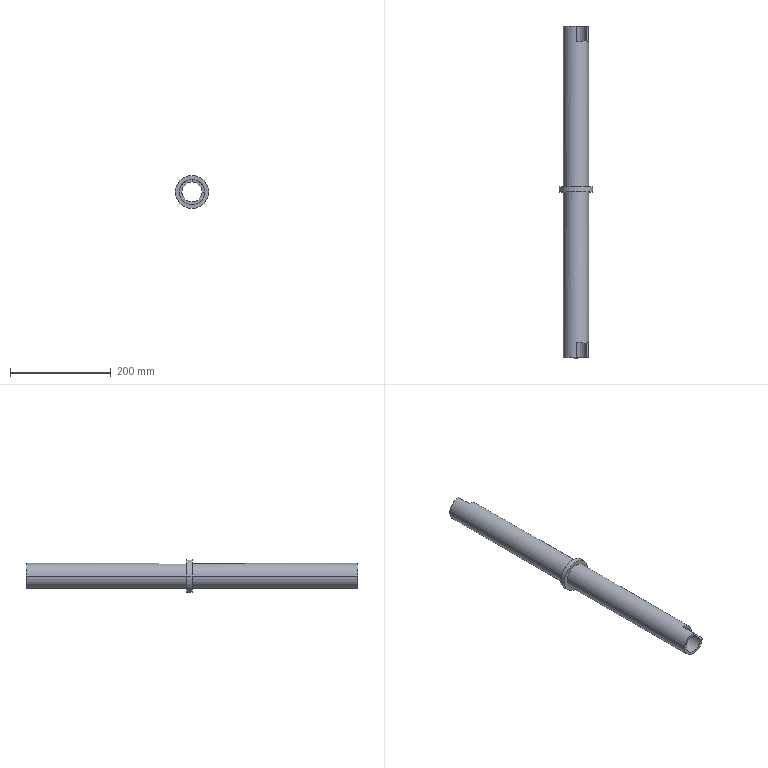Part | SolidWorks | features ICE 3, Revolution 1 | 1 solid | 18 faces | box 66 x 660 x 66 mm | volume 470501 mm3 | plane 10 | cylinder 8 | commonest cylinder face diameters 50 x4 40 x2 66 x2
STEP:
#1=CARTESIAN_POINT('',(20.,0.,0.));
#2=VERTEX_POINT('',#1);
#3=CARTESIAN_POINT('',(20.,30.,0.));
#4=VERTEX_POINT('',#3);
#5=CARTESIAN_POINT('',(20.,-0.001,0.));
#6=DIRECTION('',(0.,1.,0.));
#7=VECTOR('',#6,1000.);
#8=LINE('',#5,#7);
#9=EDGE_CURVE('',#2,#4,#8,.T.);
#10=ORIENTED_EDGE('',*,*,#9,.T.);
#11=CARTESIAN_POINT('',(20.,630.,0.));
#12=VERTEX_POINT('',#11);
#13=CARTESIAN_POINT('',(20.,-0.001,0.));
#14=DIRECTION('',(0.,1.,0.));
#15=VECTOR('',#14,1000.);
#16=LINE('',#13,#15);
#17=EDGE_CURVE('',#4,#12,#16,.T.);
#18=ORIENTED_EDGE('',*,*,#17,.T.);
#19=CARTESIAN_POINT('',(20.,660.,0.));
#20=VERTEX_POINT('',#19);
#21=CARTESIAN_POINT('',(20.,-0.001,0.));
#22=DIRECTION('',(0.,1.,0.));
#23=VECTOR('',#22,1000.);
#24=LINE('',#21,#23);
#25=EDGE_CURVE('',#12,#20,#24,.T.);
#26=ORIENTED_EDGE('',*,*,#25,.T.);
#27=CARTESIAN_POINT('',(-20.,660.,0.));
#28=VERTEX_POINT('',#27);
#29=CARTESIAN_POINT('',(0.,660.,0.));
#30=DIRECTION('',(0.,1.,0.));
#31=DIRECTION('',(-1.,0.,0.));
#32=AXIS2_PLACEMENT_3D('',#29,#30,#31);
#33=CIRCLE('',#32,20.);
#34=EDGE_CURVE('',#20,#28,#33,.T.);
#35=ORIENTED_EDGE('',*,*,#34,.T.);
#36=CARTESIAN_POINT('',(-20.,0.,0.));
#37=VERTEX_POINT('',#36);
#38=CARTESIAN_POINT('',(-20.,-0.001,0.));
#39=DIRECTION('',(0.,1.,0.));
#40=VECTOR('',#39,1000.);
#41=LINE('',#38,#40);
#42=EDGE_CURVE('',#37,#28,#41,.T.);
#43=ORIENTED_EDGE('',*,*,#42,.F.);
#44=CARTESIAN_POINT('',(0.,0.,0.));
#45=DIRECTION('',(0.,-1.,0.));
#46=DIRECTION('',(-1.,0.,0.));
#47=AXIS2_PLACEMENT_3D('',#44,#45,#46);
#48=CIRCLE('',#47,20.);
#49=EDGE_CURVE('',#37,#2,#48,.T.);
#50=ORIENTED_EDGE('',*,*,#49,.T.);
#51=EDGE_LOOP('',(#10,#18,#26,#35,#43,#50));
#52=FACE_OUTER_BOUND('',#51,.T.);
#53=CARTESIAN_POINT('',(0.,-0.001,0.));
#54=DIRECTION('',(0.,1.,0.));
#55=DIRECTION('',(-1.,0.,0.));
#56=AXIS2_PLACEMENT_3D('',#53,#54,#55);
#57=CYLINDRICAL_SURFACE('',#56,20.);
#58=ADVANCED_FACE('',(#52),#57,.F.);
#59=CARTESIAN_POINT('',(-25.,340.,0.));
#60=VERTEX_POINT('',#59);
#61=CARTESIAN_POINT('',(25.,340.,0.));
#62=VERTEX_POINT('',#61);
#63=CARTESIAN_POINT('',(0.,340.,0.));
#64=DIRECTION('',(0.,1.,0.));
#65=DIRECTION('',(-1.,0.,0.));
#66=AXIS2_PLACEMENT_3D('',#63,#64,#65);
#67=CIRCLE('',#66,25.);
#68=EDGE_CURVE('',#60,#62,#67,.T.);
#69=ORIENTED_EDGE('',*,*,#68,.T.);
#70=CARTESIAN_POINT('',(25.,630.,0.));
#71=VERTEX_POINT('',#70);
#72=CARTESIAN_POINT('',(25.,660.,0.));
#73=DIRECTION('',(0.,1.,0.));
#74=VECTOR('',#73,1000.);
#75=LINE('',#72,#74);
#76=EDGE_CURVE('',#62,#71,#75,.T.);
#77=ORIENTED_EDGE('',*,*,#76,.T.);
#78=CARTESIAN_POINT('',(0.,630.,25.));
#79=VERTEX_POINT('',#78);
#80=CARTESIAN_POINT('',(0.,630.,0.));
#81=DIRECTION('',(0.,-1.,0.));
#82=DIRECTION('',(1.,0.,0.));
#83=AXIS2_PLACEMENT_3D('',#80,#81,#82);
#84=CIRCLE('',#83,25.);
#85=EDGE_CURVE('',#71,#79,#84,.T.);
#86=ORIENTED_EDGE('',*,*,#85,.T.);
#87=CARTESIAN_POINT('',(0.,660.,25.));
#88=VERTEX_POINT('',#87);
#89=CARTESIAN_POINT('',(0.,660.,25.));
#90=DIRECTION('',(0.,1.,0.));
#91=VECTOR('',#90,1000.);
#92=LINE('',#89,#91);
#93=EDGE_CURVE('',#79,#88,#92,.T.);
#94=ORIENTED_EDGE('',*,*,#93,.T.);
#95=CARTESIAN_POINT('',(-25.,660.,0.));
#96=VERTEX_POINT('',#95);
#97=CARTESIAN_POINT('',(0.,660.,0.));
#98=DIRECTION('',(0.,1.,0.));
#99=DIRECTION('',(-1.,0.,0.));
#100=AXIS2_PLACEMENT_3D('',#97,#98,#99);
#101=CIRCLE('',#100,25.);
#102=EDGE_CURVE('',#96,#88,#101,.T.);
#103=ORIENTED_EDGE('',*,*,#102,.F.);
#104=CARTESIAN_POINT('',(-25.,660.,0.));
#105=DIRECTION('',(0.,1.,0.));
#106=VECTOR('',#105,1000.);
#107=LINE('',#104,#106);
#108=EDGE_CURVE('',#60,#96,#107,.T.);
#109=ORIENTED_EDGE('',*,*,#108,.F.);
#110=EDGE_LOOP('',(#69,#77,#86,#94,#103,#109));
#111=FACE_OUTER_BOUND('',#110,.T.);
#112=CARTESIAN_POINT('',(0.,660.,0.));
#113=DIRECTION('',(0.,1.,0.));
#114=DIRECTION('',(-1.,0.,0.));
#115=AXIS2_PLACEMENT_3D('',#112,#113,#114);
#116=CYLINDRICAL_SURFACE('',#115,25.);
#117=ADVANCED_FACE('',(#111),#116,.T.);
#118=CARTESIAN_POINT('',(-33.,330.,0.));
#119=VERTEX_POINT('',#118);
#120=CARTESIAN_POINT('',(33.,330.,0.));
#121=VERTEX_POINT('',#120);
#122=CARTESIAN_POINT('',(0.,330.,0.));
#123=DIRECTION('',(0.,1.,0.));
#124=DIRECTION('',(-1.,0.,0.));
#125=AXIS2_PLACEMENT_3D('',#122,#123,#124);
#126=CIRCLE('',#125,33.);
#127=EDGE_CURVE('',#119,#121,#126,.T.);
#128=ORIENTED_EDGE('',*,*,#127,.T.);
#129=CARTESIAN_POINT('',(33.,340.,0.));
#130=VERTEX_POINT('',#129);
#131=CARTESIAN_POINT('',(33.,660.,0.));
#132=DIRECTION('',(0.,1.,0.));
#133=VECTOR('',#132,1000.);
#134=LINE('',#131,#133);
#135=EDGE_CURVE('',#121,#130,#134,.T.);
#136=ORIENTED_EDGE('',*,*,#135,.T.);
#137=CARTESIAN_POINT('',(-33.,340.,0.));
#138=VERTEX_POINT('',#137);
#139=CARTESIAN_POINT('',(0.,340.,0.));
#140=DIRECTION('',(0.,1.,0.));
#141=DIRECTION('',(-1.,0.,0.));
#142=AXIS2_PLACEMENT_3D('',#139,#140,#141);
#143=CIRCLE('',#142,33.);
#144=EDGE_CURVE('',#138,#130,#143,.T.);
#145=ORIENTED_EDGE('',*,*,#144,.F.);
#146=CARTESIAN_POINT('',(-33.,660.,0.));
#147=DIRECTION('',(0.,1.,0.));
#148=VECTOR('',#147,1000.);
#149=LINE('',#146,#148);
#150=EDGE_CURVE('',#119,#138,#149,.T.);
#151=ORIENTED_EDGE('',*,*,#150,.F.);
#152=EDGE_LOOP('',(#128,#136,#145,#151));
#153=FACE_OUTER_BOUND('',#152,.T.);
#154=CARTESIAN_POINT('',(0.,660.,0.));
#155=DIRECTION('',(0.,1.,0.));
#156=DIRECTION('',(-1.,0.,0.));
#157=AXIS2_PLACEMENT_3D('',#154,#155,#156);
#158=CYLINDRICAL_SURFACE('',#157,33.);
#159=ADVANCED_FACE('',(#153),#158,.T.);
#160=CARTESIAN_POINT('',(25.,30.,0.));
#161=VERTEX_POINT('',#160);
#162=CARTESIAN_POINT('',(0.,30.,25.));
#163=VERTEX_POINT('',#162);
#164=CARTESIAN_POINT('',(0.,30.,0.));
#165=DIRECTION('',(0.,-1.,0.));
#166=DIRECTION('',(1.,0.,0.));
#167=AXIS2_PLACEMENT_3D('',#164,#165,#166);
#168=CIRCLE('',#167,25.);
#169=EDGE_CURVE('',#161,#163,#168,.T.);
#170=ORIENTED_EDGE('',*,*,#169,.F.);
#171=CARTESIAN_POINT('',(25.,330.,0.));
#172=VERTEX_POINT('',#171);
#173=CARTESIAN_POINT('',(25.,660.,0.));
#174=DIRECTION('',(0.,1.,0.));
#175=VECTOR('',#174,1000.);
#176=LINE('',#173,#175);
#177=EDGE_CURVE('',#161,#172,#176,.T.);
#178=ORIENTED_EDGE('',*,*,#177,.T.);
#179=CARTESIAN_POINT('',(-25.,330.,0.));
#180=VERTEX_POINT('',#179);
#181=CARTESIAN_POINT('',(0.,330.,0.));
#182=DIRECTION('',(0.,1.,0.));
#183=DIRECTION('',(-1.,0.,0.));
#184=AXIS2_PLACEMENT_3D('',#181,#182,#183);
#185=CIRCLE('',#184,25.);
#186=EDGE_CURVE('',#180,#172,#185,.T.);
#187=ORIENTED_EDGE('',*,*,#186,.F.);
#188=CARTESIAN_POINT('',(-25.,0.,0.));
#189=VERTEX_POINT('',#188);
#190=CARTESIAN_POINT('',(-25.,660.,0.));
#191=DIRECTION('',(0.,1.,0.));
#192=VECTOR('',#191,1000.);
#193=LINE('',#190,#192);
#194=EDGE_CURVE('',#189,#180,#193,.T.);
#195=ORIENTED_EDGE('',*,*,#194,.F.);
#196=CARTESIAN_POINT('',(0.,0.,25.));
#197=VERTEX_POINT('',#196);
#198=CARTESIAN_POINT('',(0.,0.,0.));
#199=DIRECTION('',(0.,1.,0.));
#200=DIRECTION('',(-1.,0.,0.));
#201=AXIS2_PLACEMENT_3D('',#198,#199,#200);
#202=CIRCLE('',#201,25.);
#203=EDGE_CURVE('',#189,#197,#202,.T.);
#204=ORIENTED_EDGE('',*,*,#203,.T.);
#205=CARTESIAN_POINT('',(0.,660.,25.));
#206=DIRECTION('',(0.,1.,0.));
#207=VECTOR('',#206,1000.);
#208=LINE('',#205,#207);
#209=EDGE_CURVE('',#197,#163,#208,.T.);
#210=ORIENTED_EDGE('',*,*,#209,.T.);
#211=EDGE_LOOP('',(#170,#178,#187,#195,#204,#210));
#212=FACE_OUTER_BOUND('',#211,.T.);
#213=CARTESIAN_POINT('',(0.,660.,0.));
#214=DIRECTION('',(0.,1.,0.));
#215=DIRECTION('',(-1.,0.,0.));
#216=AXIS2_PLACEMENT_3D('',#213,#214,#215);
#217=CYLINDRICAL_SURFACE('',#216,25.);
#218=ADVANCED_FACE('',(#212),#217,.T.);
#219=CARTESIAN_POINT('',(0.,0.,20.));
#220=VERTEX_POINT('',#219);
#221=CARTESIAN_POINT('',(0.,0.,0.));
#222=DIRECTION('',(0.,-1.,0.));
#223=DIRECTION('',(-1.,0.,0.));
#224=AXIS2_PLACEMENT_3D('',#221,#222,#223);
#225=CIRCLE('',#224,20.);
#226=EDGE_CURVE('',#220,#37,#225,.T.);
#227=ORIENTED_EDGE('',*,*,#226,.F.);
#228=CARTESIAN_POINT('',(0.,0.,0.));
#229=DIRECTION('',(0.,0.,-1.));
#230=VECTOR('',#229,1000.);
#231=LINE('',#228,#230);
#232=EDGE_CURVE('',#197,#220,#231,.T.);
#233=ORIENTED_EDGE('',*,*,#232,.F.);
#234=ORIENTED_EDGE('',*,*,#203,.F.);
#235=CARTESIAN_POINT('',(25.,0.,0.));
#236=VERTEX_POINT('',#235);
#237=CARTESIAN_POINT('',(0.,0.,0.));
#238=DIRECTION('',(0.,1.,0.));
#239=DIRECTION('',(-1.,0.,0.));
#240=AXIS2_PLACEMENT_3D('',#237,#238,#239);
#241=CIRCLE('',#240,25.);
#242=EDGE_CURVE('',#236,#189,#241,.T.);
#243=ORIENTED_EDGE('',*,*,#242,.F.);
#244=CARTESIAN_POINT('',(51.068,0.,0.));
#245=DIRECTION('',(1.,0.,0.));
#246=VECTOR('',#245,1000.);
#247=LINE('',#244,#246);
#248=EDGE_CURVE('',#2,#236,#247,.T.);
#249=ORIENTED_EDGE('',*,*,#248,.F.);
#250=ORIENTED_EDGE('',*,*,#49,.F.);
#251=EDGE_LOOP('',(#227,#233,#234,#243,#249,#250));
#252=FACE_OUTER_BOUND('',#251,.T.);
#253=CARTESIAN_POINT('',(0.,0.,0.));
#254=DIRECTION('',(0.,1.,0.));
#255=DIRECTION('',(-1.,0.,0.));
#256=AXIS2_PLACEMENT_3D('',#253,#254,#255);
#257=PLANE('',#256);
#258=ADVANCED_FACE('',(#252),#257,.F.);
#259=ORIENTED_EDGE('',*,*,#177,.F.);
#260=CARTESIAN_POINT('',(25.,660.,0.));
#261=DIRECTION('',(0.,-1.,0.));
#262=VECTOR('',#261,1000.);
#263=LINE('',#260,#262);
#264=EDGE_CURVE('',#161,#236,#263,.T.);
#265=ORIENTED_EDGE('',*,*,#264,.T.);
#266=ORIENTED_EDGE('',*,*,#242,.T.);
#267=ORIENTED_EDGE('',*,*,#194,.T.);
#268=CARTESIAN_POINT('',(0.,330.,0.));
#269=DIRECTION('',(0.,1.,0.));
#270=DIRECTION('',(-1.,0.,0.));
#271=AXIS2_PLACEMENT_3D('',#268,#269,#270);
#272=CIRCLE('',#271,25.);
#273=EDGE_CURVE('',#172,#180,#272,.T.);
#274=ORIENTED_EDGE('',*,*,#273,.F.);
#275=EDGE_LOOP('',(#259,#265,#266,#267,#274));
#276=FACE_OUTER_BOUND('',#275,.T.);
#277=CARTESIAN_POINT('',(0.,660.,0.));
#278=DIRECTION('',(0.,1.,0.));
#279=DIRECTION('',(-1.,0.,0.));
#280=AXIS2_PLACEMENT_3D('',#277,#278,#279);
#281=CYLINDRICAL_SURFACE('',#280,25.);
#282=ADVANCED_FACE('',(#276),#281,.T.);
#283=ORIENTED_EDGE('',*,*,#127,.F.);
#284=CARTESIAN_POINT('',(0.,330.,0.));
#285=DIRECTION('',(0.,1.,0.));
#286=DIRECTION('',(-1.,0.,0.));
#287=AXIS2_PLACEMENT_3D('',#284,#285,#286);
#288=CIRCLE('',#287,33.);
#289=EDGE_CURVE('',#121,#119,#288,.T.);
#290=ORIENTED_EDGE('',*,*,#289,.F.);
#291=EDGE_LOOP('',(#283,#290));
#292=FACE_OUTER_BOUND('',#291,.T.);
#293=ORIENTED_EDGE('',*,*,#186,.T.);
#294=ORIENTED_EDGE('',*,*,#273,.T.);
#295=EDGE_LOOP('',(#293,#294));
#296=FACE_BOUND('',#295,.T.);
#297=CARTESIAN_POINT('',(25.,330.,0.));
#298=DIRECTION('',(0.,1.,0.));
#299=DIRECTION('',(-1.,0.,0.));
#300=AXIS2_PLACEMENT_3D('',#297,#298,#299);
#301=PLANE('',#300);
#302=ADVANCED_FACE('',(#292,#296),#301,.F.);
#303=ORIENTED_EDGE('',*,*,#135,.F.);
#304=ORIENTED_EDGE('',*,*,#289,.T.);
#305=ORIENTED_EDGE('',*,*,#150,.T.);
#306=CARTESIAN_POINT('',(0.,340.,0.));
#307=DIRECTION('',(0.,1.,0.));
#308=DIRECTION('',(-1.,0.,0.));
#309=AXIS2_PLACEMENT_3D('',#306,#307,#308);
#310=CIRCLE('',#309,33.);
#311=EDGE_CURVE('',#130,#138,#310,.T.);
#312=ORIENTED_EDGE('',*,*,#311,.F.);
#313=EDGE_LOOP('',(#303,#304,#305,#312));
#314=FACE_OUTER_BOUND('',#313,.T.);
#315=CARTESIAN_POINT('',(0.,660.,0.));
#316=DIRECTION('',(0.,1.,0.));
#317=DIRECTION('',(-1.,0.,0.));
#318=AXIS2_PLACEMENT_3D('',#315,#316,#317);
#319=CYLINDRICAL_SURFACE('',#318,33.);
#320=ADVANCED_FACE('',(#314),#319,.T.);
#321=ORIENTED_EDGE('',*,*,#68,.F.);
#322=CARTESIAN_POINT('',(0.,340.,0.));
#323=DIRECTION('',(0.,1.,0.));
#324=DIRECTION('',(-1.,0.,0.));
#325=AXIS2_PLACEMENT_3D('',#322,#323,#324);
#326=CIRCLE('',#325,25.);
#327=EDGE_CURVE('',#62,#60,#326,.T.);
#328=ORIENTED_EDGE('',*,*,#327,.F.);
#329=EDGE_LOOP('',(#321,#328));
#330=FACE_BOUND('',#329,.T.);
#331=ORIENTED_EDGE('',*,*,#144,.T.);
#332=ORIENTED_EDGE('',*,*,#311,.T.);
#333=EDGE_LOOP('',(#331,#332));
#334=FACE_OUTER_BOUND('',#333,.T.);
#335=CARTESIAN_POINT('',(33.,340.,0.));
#336=DIRECTION('',(0.,-1.,0.));
#337=DIRECTION('',(1.,0.,0.));
#338=AXIS2_PLACEMENT_3D('',#335,#336,#337);
#339=PLANE('',#338);
#340=ADVANCED_FACE('',(#330,#334),#339,.F.);
#341=ORIENTED_EDGE('',*,*,#76,.F.);
#342=ORIENTED_EDGE('',*,*,#327,.T.);
#343=ORIENTED_EDGE('',*,*,#108,.T.);
#344=CARTESIAN_POINT('',(25.,660.,0.));
#345=VERTEX_POINT('',#344);
#346=CARTESIAN_POINT('',(0.,660.,0.));
#347=DIRECTION('',(0.,1.,0.));
#348=DIRECTION('',(-1.,0.,0.));
#349=AXIS2_PLACEMENT_3D('',#346,#347,#348);
#350=CIRCLE('',#349,25.);
#351=EDGE_CURVE('',#345,#96,#350,.T.);
#352=ORIENTED_EDGE('',*,*,#351,.F.);
#353=CARTESIAN_POINT('',(25.,660.,0.));
#354=DIRECTION('',(0.,-1.,0.));
#355=VECTOR('',#354,1000.);
#356=LINE('',#353,#355);
#357=EDGE_CURVE('',#345,#71,#356,.T.);
#358=ORIENTED_EDGE('',*,*,#357,.T.);
#359=EDGE_LOOP('',(#341,#342,#343,#352,#358));
#360=FACE_OUTER_BOUND('',#359,.T.);
#361=CARTESIAN_POINT('',(0.,660.,0.));
#362=DIRECTION('',(0.,1.,0.));
#363=DIRECTION('',(-1.,0.,0.));
#364=AXIS2_PLACEMENT_3D('',#361,#362,#363);
#365=CYLINDRICAL_SURFACE('',#364,25.);
#366=ADVANCED_FACE('',(#360),#365,.T.);
#367=ORIENTED_EDGE('',*,*,#34,.F.);
#368=CARTESIAN_POINT('',(0.,660.,0.));
#369=DIRECTION('',(-1.,0.,0.));
#370=VECTOR('',#369,1000.);
#371=LINE('',#368,#370);
#372=EDGE_CURVE('',#345,#20,#371,.T.);
#373=ORIENTED_EDGE('',*,*,#372,.F.);
#374=ORIENTED_EDGE('',*,*,#351,.T.);
#375=ORIENTED_EDGE('',*,*,#102,.T.);
#376=CARTESIAN_POINT('',(0.,660.,20.));
#377=VERTEX_POINT('',#376);
#378=CARTESIAN_POINT('',(0.,660.,43.202));
#379=DIRECTION('',(0.,0.,1.));
#380=VECTOR('',#379,1000.);
#381=LINE('',#378,#380);
#382=EDGE_CURVE('',#377,#88,#381,.T.);
#383=ORIENTED_EDGE('',*,*,#382,.F.);
#384=CARTESIAN_POINT('',(0.,660.,0.));
#385=DIRECTION('',(0.,1.,0.));
#386=DIRECTION('',(-1.,0.,0.));
#387=AXIS2_PLACEMENT_3D('',#384,#385,#386);
#388=CIRCLE('',#387,20.);
#389=EDGE_CURVE('',#28,#377,#388,.T.);
#390=ORIENTED_EDGE('',*,*,#389,.F.);
#391=EDGE_LOOP('',(#367,#373,#374,#375,#383,#390));
#392=FACE_OUTER_BOUND('',#391,.T.);
#393=CARTESIAN_POINT('',(25.,660.,0.));
#394=DIRECTION('',(0.,-1.,0.));
#395=DIRECTION('',(1.,0.,0.));
#396=AXIS2_PLACEMENT_3D('',#393,#394,#395);
#397=PLANE('',#396);
#398=ADVANCED_FACE('',(#392),#397,.F.);
#399=ORIENTED_EDGE('',*,*,#17,.F.);
#400=CARTESIAN_POINT('',(0.,30.,20.));
#401=VERTEX_POINT('',#400);
#402=CARTESIAN_POINT('',(0.,30.,0.));
#403=DIRECTION('',(0.,1.,0.));
#404=DIRECTION('',(1.,0.,0.));
#405=AXIS2_PLACEMENT_3D('',#402,#403,#404);
#406=CIRCLE('',#405,20.);
#407=EDGE_CURVE('',#401,#4,#406,.T.);
#408=ORIENTED_EDGE('',*,*,#407,.F.);
#409=CARTESIAN_POINT('',(0.,-0.001,20.));
#410=DIRECTION('',(0.,-1.,0.));
#411=VECTOR('',#410,1000.);
#412=LINE('',#409,#411);
#413=EDGE_CURVE('',#401,#220,#412,.T.);
#414=ORIENTED_EDGE('',*,*,#413,.T.);
#415=ORIENTED_EDGE('',*,*,#226,.T.);
#416=ORIENTED_EDGE('',*,*,#42,.T.);
#417=ORIENTED_EDGE('',*,*,#389,.T.);
#418=CARTESIAN_POINT('',(0.,630.,20.));
#419=VERTEX_POINT('',#418);
#420=CARTESIAN_POINT('',(0.,-0.001,20.));
#421=DIRECTION('',(0.,-1.,0.));
#422=VECTOR('',#421,1000.);
#423=LINE('',#420,#422);
#424=EDGE_CURVE('',#377,#419,#423,.T.);
#425=ORIENTED_EDGE('',*,*,#424,.T.);
#426=CARTESIAN_POINT('',(0.,630.,0.));
#427=DIRECTION('',(0.,1.,0.));
#428=DIRECTION('',(1.,0.,0.));
#429=AXIS2_PLACEMENT_3D('',#426,#427,#428);
#430=CIRCLE('',#429,20.);
#431=EDGE_CURVE('',#419,#12,#430,.T.);
#432=ORIENTED_EDGE('',*,*,#431,.T.);
#433=EDGE_LOOP('',(#399,#408,#414,#415,#416,#417,#425,#432));
#434=FACE_OUTER_BOUND('',#433,.T.);
#435=CARTESIAN_POINT('',(0.,-0.001,0.));
#436=DIRECTION('',(0.,1.,0.));
#437=DIRECTION('',(-1.,0.,0.));
#438=AXIS2_PLACEMENT_3D('',#435,#436,#437);
#439=CYLINDRICAL_SURFACE('',#438,20.);
#440=ADVANCED_FACE('',(#434),#439,.F.);
#441=ORIENTED_EDGE('',*,*,#372,.T.);
#442=ORIENTED_EDGE('',*,*,#25,.F.);
#443=CARTESIAN_POINT('',(0.,630.,0.));
#444=DIRECTION('',(-1.,0.,0.));
#445=VECTOR('',#444,1000.);
#446=LINE('',#443,#445);
#447=EDGE_CURVE('',#71,#12,#446,.T.);
#448=ORIENTED_EDGE('',*,*,#447,.F.);
#449=ORIENTED_EDGE('',*,*,#357,.F.);
#450=EDGE_LOOP('',(#441,#442,#448,#449));
#451=FACE_OUTER_BOUND('',#450,.T.);
#452=CARTESIAN_POINT('',(0.,630.,0.));
#453=DIRECTION('',(0.,0.,-1.));
#454=DIRECTION('',(-1.,0.,0.));
#455=AXIS2_PLACEMENT_3D('',#452,#453,#454);
#456=PLANE('',#455);
#457=ADVANCED_FACE('',(#451),#456,.F.);
#458=CARTESIAN_POINT('',(0.,630.,43.202));
#459=DIRECTION('',(0.,0.,1.));
#460=VECTOR('',#459,1000.);
#461=LINE('',#458,#460);
#462=EDGE_CURVE('',#419,#79,#461,.T.);
#463=ORIENTED_EDGE('',*,*,#462,.F.);
#464=ORIENTED_EDGE('',*,*,#424,.F.);
#465=ORIENTED_EDGE('',*,*,#382,.T.);
#466=ORIENTED_EDGE('',*,*,#93,.F.);
#467=EDGE_LOOP('',(#463,#464,#465,#466));
#468=FACE_OUTER_BOUND('',#467,.T.);
#469=CARTESIAN_POINT('',(0.,630.,43.202));
#470=DIRECTION('',(-1.,0.,0.));
#471=DIRECTION('',(0.,-1.,0.));
#472=AXIS2_PLACEMENT_3D('',#469,#470,#471);
#473=PLANE('',#472);
#474=ADVANCED_FACE('',(#468),#473,.F.);
#475=ORIENTED_EDGE('',*,*,#447,.T.);
#476=ORIENTED_EDGE('',*,*,#431,.F.);
#477=ORIENTED_EDGE('',*,*,#462,.T.);
#478=ORIENTED_EDGE('',*,*,#85,.F.);
#479=EDGE_LOOP('',(#475,#476,#477,#478));
#480=FACE_OUTER_BOUND('',#479,.T.);
#481=CARTESIAN_POINT('',(0.,630.,0.));
#482=DIRECTION('',(0.,-1.,0.));
#483=DIRECTION('',(1.,0.,0.));
#484=AXIS2_PLACEMENT_3D('',#481,#482,#483);
#485=PLANE('',#484);
#486=ADVANCED_FACE('',(#480),#485,.F.);
#487=ORIENTED_EDGE('',*,*,#232,.T.);
#488=ORIENTED_EDGE('',*,*,#413,.F.);
#489=CARTESIAN_POINT('',(0.,30.,0.));
#490=DIRECTION('',(0.,0.,-1.));
#491=VECTOR('',#490,1000.);
#492=LINE('',#489,#491);
#493=EDGE_CURVE('',#163,#401,#492,.T.);
#494=ORIENTED_EDGE('',*,*,#493,.F.);
#495=ORIENTED_EDGE('',*,*,#209,.F.);
#496=EDGE_LOOP('',(#487,#488,#494,#495));
#497=FACE_OUTER_BOUND('',#496,.T.);
#498=CARTESIAN_POINT('',(0.,30.,0.));
#499=DIRECTION('',(-1.,0.,0.));
#500=DIRECTION('',(0.,-1.,0.));
#501=AXIS2_PLACEMENT_3D('',#498,#499,#500);
#502=PLANE('',#501);
#503=ADVANCED_FACE('',(#497),#502,.F.);
#504=CARTESIAN_POINT('',(51.068,30.,0.));
#505=DIRECTION('',(1.,0.,0.));
#506=VECTOR('',#505,1000.);
#507=LINE('',#504,#506);
#508=EDGE_CURVE('',#4,#161,#507,.T.);
#509=ORIENTED_EDGE('',*,*,#508,.F.);
#510=ORIENTED_EDGE('',*,*,#9,.F.);
#511=ORIENTED_EDGE('',*,*,#248,.T.);
#512=ORIENTED_EDGE('',*,*,#264,.F.);
#513=EDGE_LOOP('',(#509,#510,#511,#512));
#514=FACE_OUTER_BOUND('',#513,.T.);
#515=CARTESIAN_POINT('',(51.068,30.,0.));
#516=DIRECTION('',(0.,0.,-1.));
#517=DIRECTION('',(-1.,0.,0.));
#518=AXIS2_PLACEMENT_3D('',#515,#516,#517);
#519=PLANE('',#518);
#520=ADVANCED_FACE('',(#514),#519,.F.);
#521=ORIENTED_EDGE('',*,*,#169,.T.);
#522=ORIENTED_EDGE('',*,*,#493,.T.);
#523=ORIENTED_EDGE('',*,*,#407,.T.);
#524=ORIENTED_EDGE('',*,*,#508,.T.);
#525=EDGE_LOOP('',(#521,#522,#523,#524));
#526=FACE_OUTER_BOUND('',#525,.T.);
#527=CARTESIAN_POINT('',(0.,30.,0.));
#528=DIRECTION('',(0.,-1.,0.));
#529=DIRECTION('',(1.,0.,0.));
#530=AXIS2_PLACEMENT_3D('',#527,#528,#529);
#531=PLANE('',#530);
#532=ADVANCED_FACE('',(#526),#531,.T.);
#533=CLOSED_SHELL('',(#58,#117,#159,#218,#258,#282,#302,#320,#340,#366,#398,#440,#457,#474,#486,#503,#520,#532));
#534=MANIFOLD_SOLID_BREP('',#533);
#535=CARTESIAN_POINT('',(0.,0.,0.));
#536=DIRECTION('',(0.,0.,1.));
#537=DIRECTION('',(1.,0.,0.));
#538=AXIS2_PLACEMENT_3D('',#535,#536,#537);
#539=(LENGTH_UNIT()NAMED_UNIT(*)SI_UNIT(.MILLI.,.METRE.));
#540=UNCERTAINTY_MEASURE_WITH_UNIT(LENGTH_MEASURE(0.00001),#539,'','');
#541=(NAMED_UNIT(*)PLANE_ANGLE_UNIT()SI_UNIT($,.RADIAN.));
#542=(NAMED_UNIT(*)SI_UNIT($,.STERADIAN.)SOLID_ANGLE_UNIT());
#543=(GEOMETRIC_REPRESENTATION_CONTEXT(3)GLOBAL_UNCERTAINTY_ASSIGNED_CONTEXT((#540))GLOBAL_UNIT_ASSIGNED_CONTEXT((#539,#541,#542))REPRESENTATION_CONTEXT('',''));
#544=ADVANCED_BREP_SHAPE_REPRESENTATION('',(#534,#538),#543);